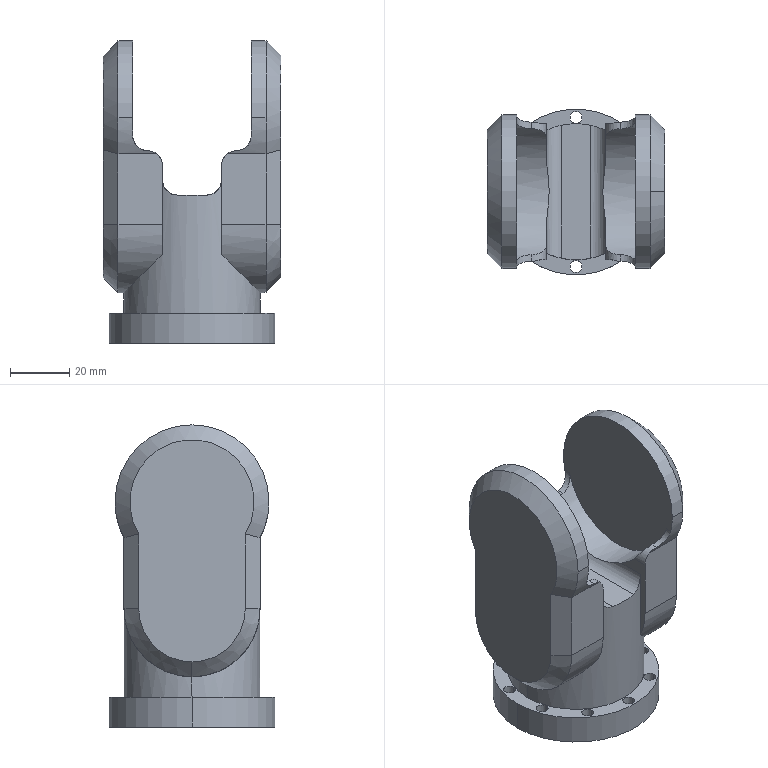Part | SolidWorks | features Cut 3, ICE 2, Chamfer 1, CirPattern 1, Extrusion 1, Fillet 1, MirrorPattern 1 | 1 solid | 69 faces | box 60 x 56 x 102.088 mm | volume 164993 mm3 | cylinder 44 | plane 19 | cone 6 | commonest cylinder face diameters 4 x20 10 x10 52 x6 46 x4 48 x2 56 x2